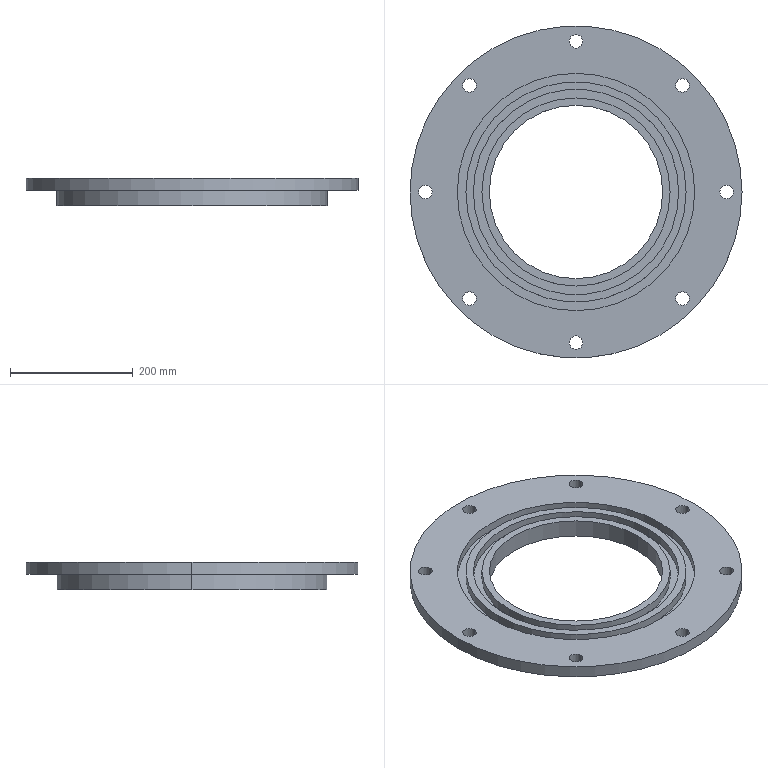Part | SolidWorks | features CirPattern 1, ICE 1, Revolution 1 | 1 solid | 40 faces | box 540 x 540 x 45 mm | volume 4136152 mm3 | cylinder 32 | plane 8 | commonest cylinder face diameters 22 x16 282 x2 306 x2 334 x2 358 x2 386 x2
STEP:
#1=CARTESIAN_POINT('',(-256.,0.,-20.));
#2=VERTEX_POINT('',#1);
#3=CARTESIAN_POINT('',(-234.,0.,-20.));
#4=VERTEX_POINT('',#3);
#5=CARTESIAN_POINT('',(-245.,0.,-20.));
#6=DIRECTION('',(0.,0.,1.));
#7=DIRECTION('',(1.,0.,0.));
#8=AXIS2_PLACEMENT_3D('',#5,#6,#7);
#9=CIRCLE('',#8,11.);
#10=EDGE_CURVE('',#2,#4,#9,.T.);
#11=ORIENTED_EDGE('',*,*,#10,.F.);
#12=CARTESIAN_POINT('',(-256.,0.,0.));
#13=VERTEX_POINT('',#12);
#14=CARTESIAN_POINT('',(-256.,0.,-41.));
#15=DIRECTION('',(0.,0.,1.));
#16=VECTOR('',#15,1000.);
#17=LINE('',#14,#16);
#18=EDGE_CURVE('',#2,#13,#17,.T.);
#19=ORIENTED_EDGE('',*,*,#18,.T.);
#20=CARTESIAN_POINT('',(-234.,0.,0.));
#21=VERTEX_POINT('',#20);
#22=CARTESIAN_POINT('',(-245.,0.,0.));
#23=DIRECTION('',(0.,0.,1.));
#24=DIRECTION('',(0.,1.,0.));
#25=AXIS2_PLACEMENT_3D('',#22,#23,#24);
#26=CIRCLE('',#25,11.);
#27=EDGE_CURVE('',#13,#21,#26,.T.);
#28=ORIENTED_EDGE('',*,*,#27,.T.);
#29=CARTESIAN_POINT('',(-234.,0.,-41.));
#30=DIRECTION('',(0.,0.,1.));
#31=VECTOR('',#30,1000.);
#32=LINE('',#29,#31);
#33=EDGE_CURVE('',#4,#21,#32,.T.);
#34=ORIENTED_EDGE('',*,*,#33,.F.);
#35=EDGE_LOOP('',(#11,#19,#28,#34));
#36=FACE_OUTER_BOUND('',#35,.T.);
#37=CARTESIAN_POINT('',(-245.,0.,-41.));
#38=DIRECTION('',(0.,0.,1.));
#39=DIRECTION('',(1.,0.,0.));
#40=AXIS2_PLACEMENT_3D('',#37,#38,#39);
#41=CYLINDRICAL_SURFACE('',#40,11.);
#42=ADVANCED_FACE('',(#36),#41,.F.);
#43=CARTESIAN_POINT('',(-184.241,-173.241,-20.));
#44=VERTEX_POINT('',#43);
#45=CARTESIAN_POINT('',(-162.241,-173.241,-20.));
#46=VERTEX_POINT('',#45);
#47=CARTESIAN_POINT('',(-173.241,-173.241,-20.));
#48=DIRECTION('',(0.,0.,1.));
#49=DIRECTION('',(1.,0.,0.));
#50=AXIS2_PLACEMENT_3D('',#47,#48,#49);
#51=CIRCLE('',#50,11.);
#52=EDGE_CURVE('',#44,#46,#51,.T.);
#53=ORIENTED_EDGE('',*,*,#52,.F.);
#54=CARTESIAN_POINT('',(-184.241,-173.241,0.));
#55=VERTEX_POINT('',#54);
#56=CARTESIAN_POINT('',(-184.241,-173.241,-41.));
#57=DIRECTION('',(0.,0.,1.));
#58=VECTOR('',#57,1000.);
#59=LINE('',#56,#58);
#60=EDGE_CURVE('',#44,#55,#59,.T.);
#61=ORIENTED_EDGE('',*,*,#60,.T.);
#62=CARTESIAN_POINT('',(-162.241,-173.241,0.));
#63=VERTEX_POINT('',#62);
#64=CARTESIAN_POINT('',(-173.241,-173.241,0.));
#65=DIRECTION('',(0.,0.,1.));
#66=DIRECTION('',(-0.7071,0.7071,0.));
#67=AXIS2_PLACEMENT_3D('',#64,#65,#66);
#68=CIRCLE('',#67,11.);
#69=EDGE_CURVE('',#55,#63,#68,.T.);
#70=ORIENTED_EDGE('',*,*,#69,.T.);
#71=CARTESIAN_POINT('',(-162.241,-173.241,-41.));
#72=DIRECTION('',(0.,0.,1.));
#73=VECTOR('',#72,1000.);
#74=LINE('',#71,#73);
#75=EDGE_CURVE('',#46,#63,#74,.T.);
#76=ORIENTED_EDGE('',*,*,#75,.F.);
#77=EDGE_LOOP('',(#53,#61,#70,#76));
#78=FACE_OUTER_BOUND('',#77,.T.);
#79=CARTESIAN_POINT('',(-173.241,-173.241,-41.));
#80=DIRECTION('',(0.,0.,1.));
#81=DIRECTION('',(1.,0.,0.));
#82=AXIS2_PLACEMENT_3D('',#79,#80,#81);
#83=CYLINDRICAL_SURFACE('',#82,11.);
#84=ADVANCED_FACE('',(#78),#83,.F.);
#85=CARTESIAN_POINT('',(-11.,-245.,-20.));
#86=VERTEX_POINT('',#85);
#87=CARTESIAN_POINT('',(11.,-245.,-20.));
#88=VERTEX_POINT('',#87);
#89=CARTESIAN_POINT('',(0.,-245.,-20.));
#90=DIRECTION('',(0.,0.,1.));
#91=DIRECTION('',(1.,0.,0.));
#92=AXIS2_PLACEMENT_3D('',#89,#90,#91);
#93=CIRCLE('',#92,11.);
#94=EDGE_CURVE('',#86,#88,#93,.T.);
#95=ORIENTED_EDGE('',*,*,#94,.F.);
#96=CARTESIAN_POINT('',(-11.,-245.,0.));
#97=VERTEX_POINT('',#96);
#98=CARTESIAN_POINT('',(-11.,-245.,-41.));
#99=DIRECTION('',(0.,0.,1.));
#100=VECTOR('',#99,1000.);
#101=LINE('',#98,#100);
#102=EDGE_CURVE('',#86,#97,#101,.T.);
#103=ORIENTED_EDGE('',*,*,#102,.T.);
#104=CARTESIAN_POINT('',(11.,-245.,0.));
#105=VERTEX_POINT('',#104);
#106=CARTESIAN_POINT('',(0.,-245.,0.));
#107=DIRECTION('',(0.,0.,1.));
#108=DIRECTION('',(-1.,0.,0.));
#109=AXIS2_PLACEMENT_3D('',#106,#107,#108);
#110=CIRCLE('',#109,11.);
#111=EDGE_CURVE('',#97,#105,#110,.T.);
#112=ORIENTED_EDGE('',*,*,#111,.T.);
#113=CARTESIAN_POINT('',(11.,-245.,-41.));
#114=DIRECTION('',(0.,0.,1.));
#115=VECTOR('',#114,1000.);
#116=LINE('',#113,#115);
#117=EDGE_CURVE('',#88,#105,#116,.T.);
#118=ORIENTED_EDGE('',*,*,#117,.F.);
#119=EDGE_LOOP('',(#95,#103,#112,#118));
#120=FACE_OUTER_BOUND('',#119,.T.);
#121=CARTESIAN_POINT('',(0.,-245.,-41.));
#122=DIRECTION('',(0.,0.,1.));
#123=DIRECTION('',(1.,0.,0.));
#124=AXIS2_PLACEMENT_3D('',#121,#122,#123);
#125=CYLINDRICAL_SURFACE('',#124,11.);
#126=ADVANCED_FACE('',(#120),#125,.F.);
#127=CARTESIAN_POINT('',(162.241,-173.241,-20.));
#128=VERTEX_POINT('',#127);
#129=CARTESIAN_POINT('',(184.241,-173.241,-20.));
#130=VERTEX_POINT('',#129);
#131=CARTESIAN_POINT('',(173.241,-173.241,-20.));
#132=DIRECTION('',(0.,0.,1.));
#133=DIRECTION('',(1.,0.,0.));
#134=AXIS2_PLACEMENT_3D('',#131,#132,#133);
#135=CIRCLE('',#134,11.);
#136=EDGE_CURVE('',#128,#130,#135,.T.);
#137=ORIENTED_EDGE('',*,*,#136,.F.);
#138=CARTESIAN_POINT('',(162.241,-173.241,0.));
#139=VERTEX_POINT('',#138);
#140=CARTESIAN_POINT('',(162.241,-173.241,-41.));
#141=DIRECTION('',(0.,0.,1.));
#142=VECTOR('',#141,1000.);
#143=LINE('',#140,#142);
#144=EDGE_CURVE('',#128,#139,#143,.T.);
#145=ORIENTED_EDGE('',*,*,#144,.T.);
#146=CARTESIAN_POINT('',(184.241,-173.241,0.));
#147=VERTEX_POINT('',#146);
#148=CARTESIAN_POINT('',(173.241,-173.241,0.));
#149=DIRECTION('',(0.,0.,1.));
#150=DIRECTION('',(-0.7071,-0.7071,0.));
#151=AXIS2_PLACEMENT_3D('',#148,#149,#150);
#152=CIRCLE('',#151,11.);
#153=EDGE_CURVE('',#139,#147,#152,.T.);
#154=ORIENTED_EDGE('',*,*,#153,.T.);
#155=CARTESIAN_POINT('',(184.241,-173.241,-41.));
#156=DIRECTION('',(0.,0.,1.));
#157=VECTOR('',#156,1000.);
#158=LINE('',#155,#157);
#159=EDGE_CURVE('',#130,#147,#158,.T.);
#160=ORIENTED_EDGE('',*,*,#159,.F.);
#161=EDGE_LOOP('',(#137,#145,#154,#160));
#162=FACE_OUTER_BOUND('',#161,.T.);
#163=CARTESIAN_POINT('',(173.241,-173.241,-41.));
#164=DIRECTION('',(0.,0.,1.));
#165=DIRECTION('',(1.,0.,0.));
#166=AXIS2_PLACEMENT_3D('',#163,#164,#165);
#167=CYLINDRICAL_SURFACE('',#166,11.);
#168=ADVANCED_FACE('',(#162),#167,.F.);
#169=CARTESIAN_POINT('',(234.,0.,-20.));
#170=VERTEX_POINT('',#169);
#171=CARTESIAN_POINT('',(256.,0.,-20.));
#172=VERTEX_POINT('',#171);
#173=CARTESIAN_POINT('',(245.,0.,-20.));
#174=DIRECTION('',(0.,0.,1.));
#175=DIRECTION('',(1.,0.,0.));
#176=AXIS2_PLACEMENT_3D('',#173,#174,#175);
#177=CIRCLE('',#176,11.);
#178=EDGE_CURVE('',#170,#172,#177,.T.);
#179=ORIENTED_EDGE('',*,*,#178,.F.);
#180=CARTESIAN_POINT('',(234.,0.,0.));
#181=VERTEX_POINT('',#180);
#182=CARTESIAN_POINT('',(234.,0.,-41.));
#183=DIRECTION('',(0.,0.,1.));
#184=VECTOR('',#183,1000.);
#185=LINE('',#182,#184);
#186=EDGE_CURVE('',#170,#181,#185,.T.);
#187=ORIENTED_EDGE('',*,*,#186,.T.);
#188=CARTESIAN_POINT('',(256.,0.,0.));
#189=VERTEX_POINT('',#188);
#190=CARTESIAN_POINT('',(245.,0.,0.));
#191=DIRECTION('',(0.,0.,1.));
#192=DIRECTION('',(0.,-1.,0.));
#193=AXIS2_PLACEMENT_3D('',#190,#191,#192);
#194=CIRCLE('',#193,11.);
#195=EDGE_CURVE('',#181,#189,#194,.T.);
#196=ORIENTED_EDGE('',*,*,#195,.T.);
#197=CARTESIAN_POINT('',(256.,0.,-41.));
#198=DIRECTION('',(0.,0.,1.));
#199=VECTOR('',#198,1000.);
#200=LINE('',#197,#199);
#201=EDGE_CURVE('',#172,#189,#200,.T.);
#202=ORIENTED_EDGE('',*,*,#201,.F.);
#203=EDGE_LOOP('',(#179,#187,#196,#202));
#204=FACE_OUTER_BOUND('',#203,.T.);
#205=CARTESIAN_POINT('',(245.,0.,-41.));
#206=DIRECTION('',(0.,0.,1.));
#207=DIRECTION('',(1.,0.,0.));
#208=AXIS2_PLACEMENT_3D('',#205,#206,#207);
#209=CYLINDRICAL_SURFACE('',#208,11.);
#210=ADVANCED_FACE('',(#204),#209,.F.);
#211=CARTESIAN_POINT('',(162.241,173.241,-20.));
#212=VERTEX_POINT('',#211);
#213=CARTESIAN_POINT('',(184.241,173.241,-20.));
#214=VERTEX_POINT('',#213);
#215=CARTESIAN_POINT('',(173.241,173.241,-20.));
#216=DIRECTION('',(0.,0.,1.));
#217=DIRECTION('',(1.,0.,0.));
#218=AXIS2_PLACEMENT_3D('',#215,#216,#217);
#219=CIRCLE('',#218,11.);
#220=EDGE_CURVE('',#212,#214,#219,.T.);
#221=ORIENTED_EDGE('',*,*,#220,.F.);
#222=CARTESIAN_POINT('',(162.241,173.241,0.));
#223=VERTEX_POINT('',#222);
#224=CARTESIAN_POINT('',(162.241,173.241,-41.));
#225=DIRECTION('',(0.,0.,1.));
#226=VECTOR('',#225,1000.);
#227=LINE('',#224,#226);
#228=EDGE_CURVE('',#212,#223,#227,.T.);
#229=ORIENTED_EDGE('',*,*,#228,.T.);
#230=CARTESIAN_POINT('',(184.241,173.241,0.));
#231=VERTEX_POINT('',#230);
#232=CARTESIAN_POINT('',(173.241,173.241,0.));
#233=DIRECTION('',(0.,0.,1.));
#234=DIRECTION('',(0.7071,-0.7071,0.));
#235=AXIS2_PLACEMENT_3D('',#232,#233,#234);
#236=CIRCLE('',#235,11.);
#237=EDGE_CURVE('',#223,#231,#236,.T.);
#238=ORIENTED_EDGE('',*,*,#237,.T.);
#239=CARTESIAN_POINT('',(184.241,173.241,-41.));
#240=DIRECTION('',(0.,0.,1.));
#241=VECTOR('',#240,1000.);
#242=LINE('',#239,#241);
#243=EDGE_CURVE('',#214,#231,#242,.T.);
#244=ORIENTED_EDGE('',*,*,#243,.F.);
#245=EDGE_LOOP('',(#221,#229,#238,#244));
#246=FACE_OUTER_BOUND('',#245,.T.);
#247=CARTESIAN_POINT('',(173.241,173.241,-41.));
#248=DIRECTION('',(0.,0.,1.));
#249=DIRECTION('',(1.,0.,0.));
#250=AXIS2_PLACEMENT_3D('',#247,#248,#249);
#251=CYLINDRICAL_SURFACE('',#250,11.);
#252=ADVANCED_FACE('',(#246),#251,.F.);
#253=CARTESIAN_POINT('',(-184.241,173.241,-20.));
#254=VERTEX_POINT('',#253);
#255=CARTESIAN_POINT('',(-162.241,173.241,-20.));
#256=VERTEX_POINT('',#255);
#257=CARTESIAN_POINT('',(-173.241,173.241,-20.));
#258=DIRECTION('',(0.,0.,1.));
#259=DIRECTION('',(1.,0.,0.));
#260=AXIS2_PLACEMENT_3D('',#257,#258,#259);
#261=CIRCLE('',#260,11.);
#262=EDGE_CURVE('',#254,#256,#261,.T.);
#263=ORIENTED_EDGE('',*,*,#262,.F.);
#264=CARTESIAN_POINT('',(-184.241,173.241,0.));
#265=VERTEX_POINT('',#264);
#266=CARTESIAN_POINT('',(-184.241,173.241,-41.));
#267=DIRECTION('',(0.,0.,1.));
#268=VECTOR('',#267,1000.);
#269=LINE('',#266,#268);
#270=EDGE_CURVE('',#254,#265,#269,.T.);
#271=ORIENTED_EDGE('',*,*,#270,.T.);
#272=CARTESIAN_POINT('',(-162.241,173.241,0.));
#273=VERTEX_POINT('',#272);
#274=CARTESIAN_POINT('',(-173.241,173.241,0.));
#275=DIRECTION('',(0.,0.,1.));
#276=DIRECTION('',(0.7071,0.7071,0.));
#277=AXIS2_PLACEMENT_3D('',#274,#275,#276);
#278=CIRCLE('',#277,11.);
#279=EDGE_CURVE('',#265,#273,#278,.T.);
#280=ORIENTED_EDGE('',*,*,#279,.T.);
#281=CARTESIAN_POINT('',(-162.241,173.241,-41.));
#282=DIRECTION('',(0.,0.,1.));
#283=VECTOR('',#282,1000.);
#284=LINE('',#281,#283);
#285=EDGE_CURVE('',#256,#273,#284,.T.);
#286=ORIENTED_EDGE('',*,*,#285,.F.);
#287=EDGE_LOOP('',(#263,#271,#280,#286));
#288=FACE_OUTER_BOUND('',#287,.T.);
#289=CARTESIAN_POINT('',(-173.241,173.241,-41.));
#290=DIRECTION('',(0.,0.,1.));
#291=DIRECTION('',(1.,0.,0.));
#292=AXIS2_PLACEMENT_3D('',#289,#290,#291);
#293=CYLINDRICAL_SURFACE('',#292,11.);
#294=ADVANCED_FACE('',(#288),#293,.F.);
#295=CARTESIAN_POINT('',(-11.,245.,-20.));
#296=VERTEX_POINT('',#295);
#297=CARTESIAN_POINT('',(11.,245.,-20.));
#298=VERTEX_POINT('',#297);
#299=CARTESIAN_POINT('',(0.,245.,-20.));
#300=DIRECTION('',(0.,0.,1.));
#301=DIRECTION('',(1.,0.,0.));
#302=AXIS2_PLACEMENT_3D('',#299,#300,#301);
#303=CIRCLE('',#302,11.);
#304=EDGE_CURVE('',#296,#298,#303,.T.);
#305=ORIENTED_EDGE('',*,*,#304,.F.);
#306=CARTESIAN_POINT('',(-11.,245.,0.));
#307=VERTEX_POINT('',#306);
#308=CARTESIAN_POINT('',(-11.,245.,-41.));
#309=DIRECTION('',(0.,0.,1.));
#310=VECTOR('',#309,1000.);
#311=LINE('',#308,#310);
#312=EDGE_CURVE('',#296,#307,#311,.T.);
#313=ORIENTED_EDGE('',*,*,#312,.T.);
#314=CARTESIAN_POINT('',(11.,245.,0.));
#315=VERTEX_POINT('',#314);
#316=CARTESIAN_POINT('',(0.,245.,0.));
#317=DIRECTION('',(0.,0.,1.));
#318=DIRECTION('',(1.,0.,0.));
#319=AXIS2_PLACEMENT_3D('',#316,#317,#318);
#320=CIRCLE('',#319,11.);
#321=EDGE_CURVE('',#307,#315,#320,.T.);
#322=ORIENTED_EDGE('',*,*,#321,.T.);
#323=CARTESIAN_POINT('',(11.,245.,-41.));
#324=DIRECTION('',(0.,0.,1.));
#325=VECTOR('',#324,1000.);
#326=LINE('',#323,#325);
#327=EDGE_CURVE('',#298,#315,#326,.T.);
#328=ORIENTED_EDGE('',*,*,#327,.F.);
#329=EDGE_LOOP('',(#305,#313,#322,#328));
#330=FACE_OUTER_BOUND('',#329,.T.);
#331=CARTESIAN_POINT('',(0.,245.,-41.));
#332=DIRECTION('',(0.,0.,1.));
#333=DIRECTION('',(1.,0.,0.));
#334=AXIS2_PLACEMENT_3D('',#331,#332,#333);
#335=CYLINDRICAL_SURFACE('',#334,11.);
#336=ADVANCED_FACE('',(#330),#335,.F.);
#337=CARTESIAN_POINT('',(-193.,0.,-14.));
#338=VERTEX_POINT('',#337);
#339=CARTESIAN_POINT('',(193.,0.,-14.));
#340=VERTEX_POINT('',#339);
#341=CARTESIAN_POINT('',(0.,0.,-14.));
#342=DIRECTION('',(0.,0.,1.));
#343=DIRECTION('',(1.,0.,0.));
#344=AXIS2_PLACEMENT_3D('',#341,#342,#343);
#345=CIRCLE('',#344,193.);
#346=EDGE_CURVE('',#338,#340,#345,.T.);
#347=ORIENTED_EDGE('',*,*,#346,.F.);
#348=CARTESIAN_POINT('',(-193.,0.,0.));
#349=VERTEX_POINT('',#348);
#350=CARTESIAN_POINT('',(-193.,0.,0.));
#351=DIRECTION('',(0.,0.,1.));
#352=VECTOR('',#351,1000.);
#353=LINE('',#350,#352);
#354=EDGE_CURVE('',#338,#349,#353,.T.);
#355=ORIENTED_EDGE('',*,*,#354,.T.);
#356=CARTESIAN_POINT('',(193.,0.,0.));
#357=VERTEX_POINT('',#356);
#358=CARTESIAN_POINT('',(0.,0.,0.));
#359=DIRECTION('',(0.,0.,1.));
#360=DIRECTION('',(1.,0.,0.));
#361=AXIS2_PLACEMENT_3D('',#358,#359,#360);
#362=CIRCLE('',#361,193.);
#363=EDGE_CURVE('',#349,#357,#362,.T.);
#364=ORIENTED_EDGE('',*,*,#363,.T.);
#365=CARTESIAN_POINT('',(193.,0.,0.));
#366=DIRECTION('',(0.,0.,1.));
#367=VECTOR('',#366,1000.);
#368=LINE('',#365,#367);
#369=EDGE_CURVE('',#340,#357,#368,.T.);
#370=ORIENTED_EDGE('',*,*,#369,.F.);
#371=EDGE_LOOP('',(#347,#355,#364,#370));
#372=FACE_OUTER_BOUND('',#371,.T.);
#373=CARTESIAN_POINT('',(0.,0.,0.));
#374=DIRECTION('',(0.,0.,1.));
#375=DIRECTION('',(1.,0.,0.));
#376=AXIS2_PLACEMENT_3D('',#373,#374,#375);
#377=CYLINDRICAL_SURFACE('',#376,193.);
#378=ADVANCED_FACE('',(#372),#377,.F.);
#379=CARTESIAN_POINT('',(179.,0.,-14.));
#380=VERTEX_POINT('',#379);
#381=CARTESIAN_POINT('',(-179.,0.,-14.));
#382=VERTEX_POINT('',#381);
#383=CARTESIAN_POINT('',(0.,0.,-14.));
#384=DIRECTION('',(0.,0.,1.));
#385=DIRECTION('',(1.,0.,0.));
#386=AXIS2_PLACEMENT_3D('',#383,#384,#385);
#387=CIRCLE('',#386,179.);
#388=EDGE_CURVE('',#380,#382,#387,.T.);
#389=ORIENTED_EDGE('',*,*,#388,.T.);
#390=CARTESIAN_POINT('',(-179.,0.,0.));
#391=VERTEX_POINT('',#390);
#392=CARTESIAN_POINT('',(-179.,0.,0.));
#393=DIRECTION('',(0.,0.,1.));
#394=VECTOR('',#393,1000.);
#395=LINE('',#392,#394);
#396=EDGE_CURVE('',#382,#391,#395,.T.);
#397=ORIENTED_EDGE('',*,*,#396,.T.);
#398=CARTESIAN_POINT('',(179.,0.,0.));
#399=VERTEX_POINT('',#398);
#400=CARTESIAN_POINT('',(0.,0.,0.));
#401=DIRECTION('',(0.,0.,1.));
#402=DIRECTION('',(1.,0.,0.));
#403=AXIS2_PLACEMENT_3D('',#400,#401,#402);
#404=CIRCLE('',#403,179.);
#405=EDGE_CURVE('',#399,#391,#404,.T.);
#406=ORIENTED_EDGE('',*,*,#405,.F.);
#407=CARTESIAN_POINT('',(179.,0.,0.));
#408=DIRECTION('',(0.,0.,1.));
#409=VECTOR('',#408,1000.);
#410=LINE('',#407,#409);
#411=EDGE_CURVE('',#380,#399,#410,.T.);
#412=ORIENTED_EDGE('',*,*,#411,.F.);
#413=EDGE_LOOP('',(#389,#397,#406,#412));
#414=FACE_OUTER_BOUND('',#413,.T.);
#415=CARTESIAN_POINT('',(0.,0.,0.));
#416=DIRECTION('',(0.,0.,1.));
#417=DIRECTION('',(1.,0.,0.));
#418=AXIS2_PLACEMENT_3D('',#415,#416,#417);
#419=CYLINDRICAL_SURFACE('',#418,179.);
#420=ADVANCED_FACE('',(#414),#419,.T.);
#421=CARTESIAN_POINT('',(-167.,0.,-14.));
#422=VERTEX_POINT('',#421);
#423=CARTESIAN_POINT('',(167.,0.,-14.));
#424=VERTEX_POINT('',#423);
#425=CARTESIAN_POINT('',(0.,0.,-14.));
#426=DIRECTION('',(0.,0.,1.));
#427=DIRECTION('',(1.,0.,0.));
#428=AXIS2_PLACEMENT_3D('',#425,#426,#427);
#429=CIRCLE('',#428,167.);
#430=EDGE_CURVE('',#422,#424,#429,.T.);
#431=ORIENTED_EDGE('',*,*,#430,.F.);
#432=CARTESIAN_POINT('',(-167.,0.,0.));
#433=VERTEX_POINT('',#432);
#434=CARTESIAN_POINT('',(-167.,0.,0.));
#435=DIRECTION('',(0.,0.,1.));
#436=VECTOR('',#435,1000.);
#437=LINE('',#434,#436);
#438=EDGE_CURVE('',#422,#433,#437,.T.);
#439=ORIENTED_EDGE('',*,*,#438,.T.);
#440=CARTESIAN_POINT('',(167.,0.,0.));
#441=VERTEX_POINT('',#440);
#442=CARTESIAN_POINT('',(0.,0.,0.));
#443=DIRECTION('',(0.,0.,1.));
#444=DIRECTION('',(1.,0.,0.));
#445=AXIS2_PLACEMENT_3D('',#442,#443,#444);
#446=CIRCLE('',#445,167.);
#447=EDGE_CURVE('',#433,#441,#446,.T.);
#448=ORIENTED_EDGE('',*,*,#447,.T.);
#449=CARTESIAN_POINT('',(167.,0.,0.));
#450=DIRECTION('',(0.,0.,1.));
#451=VECTOR('',#450,1000.);
#452=LINE('',#449,#451);
#453=EDGE_CURVE('',#424,#441,#452,.T.);
#454=ORIENTED_EDGE('',*,*,#453,.F.);
#455=EDGE_LOOP('',(#431,#439,#448,#454));
#456=FACE_OUTER_BOUND('',#455,.T.);
#457=CARTESIAN_POINT('',(0.,0.,0.));
#458=DIRECTION('',(0.,0.,1.));
#459=DIRECTION('',(1.,0.,0.));
#460=AXIS2_PLACEMENT_3D('',#457,#458,#459);
#461=CYLINDRICAL_SURFACE('',#460,167.);
#462=ADVANCED_FACE('',(#456),#461,.F.);
#463=CARTESIAN_POINT('',(153.,0.,-14.));
#464=VERTEX_POINT('',#463);
#465=CARTESIAN_POINT('',(-153.,0.,-14.));
#466=VERTEX_POINT('',#465);
#467=CARTESIAN_POINT('',(0.,0.,-14.));
#468=DIRECTION('',(0.,0.,1.));
#469=DIRECTION('',(1.,0.,0.));
#470=AXIS2_PLACEMENT_3D('',#467,#468,#469);
#471=CIRCLE('',#470,153.);
#472=EDGE_CURVE('',#464,#466,#471,.T.);
#473=ORIENTED_EDGE('',*,*,#472,.T.);
#474=CARTESIAN_POINT('',(-153.,0.,0.));
#475=VERTEX_POINT('',#474);
#476=CARTESIAN_POINT('',(-153.,0.,0.));
#477=DIRECTION('',(0.,0.,1.));
#478=VECTOR('',#477,1000.);
#479=LINE('',#476,#478);
#480=EDGE_CURVE('',#466,#475,#479,.T.);
#481=ORIENTED_EDGE('',*,*,#480,.T.);
#482=CARTESIAN_POINT('',(153.,0.,0.));
#483=VERTEX_POINT('',#482);
#484=CARTESIAN_POINT('',(0.,0.,0.));
#485=DIRECTION('',(0.,0.,1.));
#486=DIRECTION('',(1.,0.,0.));
#487=AXIS2_PLACEMENT_3D('',#484,#485,#486);
#488=CIRCLE('',#487,153.);
#489=EDGE_CURVE('',#483,#475,#488,.T.);
#490=ORIENTED_EDGE('',*,*,#489,.F.);
#491=CARTESIAN_POINT('',(153.,0.,0.));
#492=DIRECTION('',(0.,0.,1.));
#493=VECTOR('',#492,1000.);
#494=LINE('',#491,#493);
#495=EDGE_CURVE('',#464,#483,#494,.T.);
#496=ORIENTED_EDGE('',*,*,#495,.F.);
#497=EDGE_LOOP('',(#473,#481,#490,#496));
#498=FACE_OUTER_BOUND('',#497,.T.);
#499=CARTESIAN_POINT('',(0.,0.,0.));
#500=DIRECTION('',(0.,0.,1.));
#501=DIRECTION('',(1.,0.,0.));
#502=AXIS2_PLACEMENT_3D('',#499,#500,#501);
#503=CYLINDRICAL_SURFACE('',#502,153.);
#504=ADVANCED_FACE('',(#498),#503,.T.);
#505=CARTESIAN_POINT('',(-141.,0.,-30.));
#506=VERTEX_POINT('',#505);
#507=CARTESIAN_POINT('',(141.,0.,-30.));
#508=VERTEX_POINT('',#507);
#509=CARTESIAN_POINT('',(0.,0.,-30.));
#510=DIRECTION('',(0.,0.,1.));
#511=DIRECTION('',(1.,0.,0.));
#512=AXIS2_PLACEMENT_3D('',#509,#510,#511);
#513=CIRCLE('',#512,141.);
#514=EDGE_CURVE('',#506,#508,#513,.T.);
#515=ORIENTED_EDGE('',*,*,#514,.F.);
#516=CARTESIAN_POINT('',(-141.,0.,0.));
#517=VERTEX_POINT('',#516);
#518=CARTESIAN_POINT('',(-141.,0.,0.));
#519=DIRECTION('',(0.,0.,1.));
#520=VECTOR('',#519,1000.);
#521=LINE('',#518,#520);
#522=EDGE_CURVE('',#506,#517,#521,.T.);
#523=ORIENTED_EDGE('',*,*,#522,.T.);
#524=CARTESIAN_POINT('',(141.,0.,0.));
#525=VERTEX_POINT('',#524);
#526=CARTESIAN_POINT('',(0.,0.,0.));
#527=DIRECTION('',(0.,0.,1.));
#528=DIRECTION('',(1.,0.,0.));
#529=AXIS2_PLACEMENT_3D('',#526,#527,#528);
#530=CIRCLE('',#529,141.);
#531=EDGE_CURVE('',#517,#525,#530,.T.);
#532=ORIENTED_EDGE('',*,*,#531,.T.);
#533=CARTESIAN_POINT('',(141.,0.,0.));
#534=DIRECTION('',(0.,0.,1.));
#535=VECTOR('',#534,1000.);
#536=LINE('',#533,#535);
#537=EDGE_CURVE('',#508,#525,#536,.T.);
#538=ORIENTED_EDGE('',*,*,#537,.F.);
#539=EDGE_LOOP('',(#515,#523,#532,#538));
#540=FACE_OUTER_BOUND('',#539,.T.);
#541=CARTESIAN_POINT('',(0.,0.,0.));
#542=DIRECTION('',(0.,0.,1.));
#543=DIRECTION('',(1.,0.,0.));
#544=AXIS2_PLACEMENT_3D('',#541,#542,#543);
#545=CYLINDRICAL_SURFACE('',#544,141.);
#546=ADVANCED_FACE('',(#540),#545,.F.);
#547=CARTESIAN_POINT('',(-200.,0.,-45.));
#548=VERTEX_POINT('',#547);
#549=CARTESIAN_POINT('',(200.,0.,-45.));
#550=VERTEX_POINT('',#549);
#551=CARTESIAN_POINT('',(0.,0.,-45.));
#552=DIRECTION('',(0.,0.,1.));
#553=DIRECTION('',(1.,0.,0.));
#554=AXIS2_PLACEMENT_3D('',#551,#552,#553);
#555=CIRCLE('',#554,200.);
#556=EDGE_CURVE('',#548,#550,#555,.T.);
#557=ORIENTED_EDGE('',*,*,#556,.F.);
#558=CARTESIAN_POINT('',(-200.,0.,-30.));
#559=VERTEX_POINT('',#558);
#560=CARTESIAN_POINT('',(-200.,0.,0.));
#561=DIRECTION('',(0.,0.,1.));
#562=VECTOR('',#561,1000.);
#563=LINE('',#560,#562);
#564=EDGE_CURVE('',#548,#559,#563,.T.);
#565=ORIENTED_EDGE('',*,*,#564,.T.);
#566=CARTESIAN_POINT('',(200.,0.,-30.));
#567=VERTEX_POINT('',#566);
#568=CARTESIAN_POINT('',(0.,0.,-30.));
#569=DIRECTION('',(0.,0.,1.));
#570=DIRECTION('',(1.,0.,0.));
#571=AXIS2_PLACEMENT_3D('',#568,#569,#570);
#572=CIRCLE('',#571,200.);
#573=EDGE_CURVE('',#559,#567,#572,.T.);
#574=ORIENTED_EDGE('',*,*,#573,.T.);
#575=CARTESIAN_POINT('',(200.,0.,0.));
#576=DIRECTION('',(0.,0.,1.));
#577=VECTOR('',#576,1000.);
#578=LINE('',#575,#577);
#579=EDGE_CURVE('',#550,#567,#578,.T.);
#580=ORIENTED_EDGE('',*,*,#579,.F.);
#581=EDGE_LOOP('',(#557,#565,#574,#580));
#582=FACE_OUTER_BOUND('',#581,.T.);
#583=CARTESIAN_POINT('',(0.,0.,0.));
#584=DIRECTION('',(0.,0.,1.));
#585=DIRECTION('',(1.,0.,0.));
#586=AXIS2_PLACEMENT_3D('',#583,#584,#585);
#587=CYLINDRICAL_SURFACE('',#586,200.);
#588=ADVANCED_FACE('',(#582),#587,.F.);
#589=CARTESIAN_POINT('',(220.,0.,-45.));
#590=VERTEX_POINT('',#589);
#591=CARTESIAN_POINT('',(-220.,0.,-45.));
#592=VERTEX_POINT('',#591);
#593=CARTESIAN_POINT('',(0.,0.,-45.));
#594=DIRECTION('',(0.,0.,1.));
#595=DIRECTION('',(1.,0.,0.));
#596=AXIS2_PLACEMENT_3D('',#593,#594,#595);
#597=CIRCLE('',#596,220.);
#598=EDGE_CURVE('',#590,#592,#597,.T.);
#599=ORIENTED_EDGE('',*,*,#598,.T.);
#600=CARTESIAN_POINT('',(-220.,0.,-20.));
#601=VERTEX_POINT('',#600);
#602=CARTESIAN_POINT('',(-220.,0.,0.));
#603=DIRECTION('',(0.,0.,1.));
#604=VECTOR('',#603,1000.);
#605=LINE('',#602,#604);
#606=EDGE_CURVE('',#592,#601,#605,.T.);
#607=ORIENTED_EDGE('',*,*,#606,.T.);
#608=CARTESIAN_POINT('',(220.,0.,-20.));
#609=VERTEX_POINT('',#608);
#610=CARTESIAN_POINT('',(0.,0.,-20.));
#611=DIRECTION('',(0.,0.,1.));
#612=DIRECTION('',(1.,0.,0.));
#613=AXIS2_PLACEMENT_3D('',#610,#611,#612);
#614=CIRCLE('',#613,220.);
#615=EDGE_CURVE('',#609,#601,#614,.T.);
#616=ORIENTED_EDGE('',*,*,#615,.F.);
#617=CARTESIAN_POINT('',(220.,0.,0.));
#618=DIRECTION('',(0.,0.,1.));
#619=VECTOR('',#618,1000.);
#620=LINE('',#617,#619);
#621=EDGE_CURVE('',#590,#609,#620,.T.);
#622=ORIENTED_EDGE('',*,*,#621,.F.);
#623=EDGE_LOOP('',(#599,#607,#616,#622));
#624=FACE_OUTER_BOUND('',#623,.T.);
#625=CARTESIAN_POINT('',(0.,0.,0.));
#626=DIRECTION('',(0.,0.,1.));
#627=DIRECTION('',(1.,0.,0.));
#628=AXIS2_PLACEMENT_3D('',#625,#626,#627);
#629=CYLINDRICAL_SURFACE('',#628,220.);
#630=ADVANCED_FACE('',(#624),#629,.T.);
#631=CARTESIAN_POINT('',(270.,0.,-20.));
#632=VERTEX_POINT('',#631);
#633=CARTESIAN_POINT('',(-270.,0.,-20.));
#634=VERTEX_POINT('',#633);
#635=CARTESIAN_POINT('',(0.,0.,-20.));
#636=DIRECTION('',(0.,0.,1.));
#637=DIRECTION('',(1.,0.,0.));
#638=AXIS2_PLACEMENT_3D('',#635,#636,#637);
#639=CIRCLE('',#638,270.);
#640=EDGE_CURVE('',#632,#634,#639,.T.);
#641=ORIENTED_EDGE('',*,*,#640,.T.);
#642=CARTESIAN_POINT('',(-270.,0.,0.));
#643=VERTEX_POINT('',#642);
#644=CARTESIAN_POINT('',(-270.,0.,0.));
#645=DIRECTION('',(0.,0.,1.));
#646=VECTOR('',#645,1000.);
#647=LINE('',#644,#646);
#648=EDGE_CURVE('',#634,#643,#647,.T.);
#649=ORIENTED_EDGE('',*,*,#648,.T.);
#650=CARTESIAN_POINT('',(270.,0.,0.));
#651=VERTEX_POINT('',#650);
#652=CARTESIAN_POINT('',(0.,0.,0.));
#653=DIRECTION('',(0.,0.,1.));
#654=DIRECTION('',(1.,0.,0.));
#655=AXIS2_PLACEMENT_3D('',#652,#653,#654);
#656=CIRCLE('',#655,270.);
#657=EDGE_CURVE('',#651,#643,#656,.T.);
#658=ORIENTED_EDGE('',*,*,#657,.F.);
#659=CARTESIAN_POINT('',(270.,0.,0.));
#660=DIRECTION('',(0.,0.,1.));
#661=VECTOR('',#660,1000.);
#662=LINE('',#659,#661);
#663=EDGE_CURVE('',#632,#651,#662,.T.);
#664=ORIENTED_EDGE('',*,*,#663,.F.);
#665=EDGE_LOOP('',(#641,#649,#658,#664));
#666=FACE_OUTER_BOUND('',#665,.T.);
#667=CARTESIAN_POINT('',(0.,0.,0.));
#668=DIRECTION('',(0.,0.,1.));
#669=DIRECTION('',(1.,0.,0.));
#670=AXIS2_PLACEMENT_3D('',#667,#668,#669);
#671=CYLINDRICAL_SURFACE('',#670,270.);
#672=ADVANCED_FACE('',(#666),#671,.T.);
#673=CARTESIAN_POINT('',(-245.,0.,0.));
#674=DIRECTION('',(0.,0.,1.));
#675=DIRECTION('',(0.,1.,0.));
#676=AXIS2_PLACEMENT_3D('',#673,#674,#675);
#677=CIRCLE('',#676,11.);
#678=EDGE_CURVE('',#21,#13,#677,.T.);
#679=ORIENTED_EDGE('',*,*,#678,.F.);
#680=ORIENTED_EDGE('',*,*,#27,.F.);
#681=EDGE_LOOP('',(#679,#680));
#682=FACE_BOUND('',#681,.T.);
#683=CARTESIAN_POINT('',(-173.241,-173.241,0.));
#684=DIRECTION('',(0.,0.,1.));
#685=DIRECTION('',(-0.7071,0.7071,0.));
#686=AXIS2_PLACEMENT_3D('',#683,#684,#685);
#687=CIRCLE('',#686,11.);
#688=EDGE_CURVE('',#63,#55,#687,.T.);
#689=ORIENTED_EDGE('',*,*,#688,.F.);
#690=ORIENTED_EDGE('',*,*,#69,.F.);
#691=EDGE_LOOP('',(#689,#690));
#692=FACE_BOUND('',#691,.T.);
#693=CARTESIAN_POINT('',(0.,-245.,0.));
#694=DIRECTION('',(0.,0.,1.));
#695=DIRECTION('',(-1.,0.,0.));
#696=AXIS2_PLACEMENT_3D('',#693,#694,#695);
#697=CIRCLE('',#696,11.);
#698=EDGE_CURVE('',#105,#97,#697,.T.);
#699=ORIENTED_EDGE('',*,*,#698,.F.);
#700=ORIENTED_EDGE('',*,*,#111,.F.);
#701=EDGE_LOOP('',(#699,#700));
#702=FACE_BOUND('',#701,.T.);
#703=CARTESIAN_POINT('',(173.241,-173.241,0.));
#704=DIRECTION('',(0.,0.,1.));
#705=DIRECTION('',(-0.7071,-0.7071,0.));
#706=AXIS2_PLACEMENT_3D('',#703,#704,#705);
#707=CIRCLE('',#706,11.);
#708=EDGE_CURVE('',#147,#139,#707,.T.);
#709=ORIENTED_EDGE('',*,*,#708,.F.);
#710=ORIENTED_EDGE('',*,*,#153,.F.);
#711=EDGE_LOOP('',(#709,#710));
#712=FACE_BOUND('',#711,.T.);
#713=CARTESIAN_POINT('',(245.,0.,0.));
#714=DIRECTION('',(0.,0.,1.));
#715=DIRECTION('',(0.,-1.,0.));
#716=AXIS2_PLACEMENT_3D('',#713,#714,#715);
#717=CIRCLE('',#716,11.);
#718=EDGE_CURVE('',#189,#181,#717,.T.);
#719=ORIENTED_EDGE('',*,*,#718,.F.);
#720=ORIENTED_EDGE('',*,*,#195,.F.);
#721=EDGE_LOOP('',(#719,#720));
#722=FACE_BOUND('',#721,.T.);
#723=CARTESIAN_POINT('',(173.241,173.241,0.));
#724=DIRECTION('',(0.,0.,1.));
#725=DIRECTION('',(0.7071,-0.7071,0.));
#726=AXIS2_PLACEMENT_3D('',#723,#724,#725);
#727=CIRCLE('',#726,11.);
#728=EDGE_CURVE('',#231,#223,#727,.T.);
#729=ORIENTED_EDGE('',*,*,#728,.F.);
#730=ORIENTED_EDGE('',*,*,#237,.F.);
#731=EDGE_LOOP('',(#729,#730));
#732=FACE_BOUND('',#731,.T.);
#733=CARTESIAN_POINT('',(-173.241,173.241,0.));
#734=DIRECTION('',(0.,0.,1.));
#735=DIRECTION('',(0.7071,0.7071,0.));
#736=AXIS2_PLACEMENT_3D('',#733,#734,#735);
#737=CIRCLE('',#736,11.);
#738=EDGE_CURVE('',#273,#265,#737,.T.);
#739=ORIENTED_EDGE('',*,*,#738,.F.);
#740=ORIENTED_EDGE('',*,*,#279,.F.);
#741=EDGE_LOOP('',(#739,#740));
#742=FACE_BOUND('',#741,.T.);
#743=CARTESIAN_POINT('',(0.,245.,0.));
#744=DIRECTION('',(0.,0.,1.));
#745=DIRECTION('',(1.,0.,0.));
#746=AXIS2_PLACEMENT_3D('',#743,#744,#745);
#747=CIRCLE('',#746,11.);
#748=EDGE_CURVE('',#315,#307,#747,.T.);
#749=ORIENTED_EDGE('',*,*,#748,.F.);
#750=ORIENTED_EDGE('',*,*,#321,.F.);
#751=EDGE_LOOP('',(#749,#750));
#752=FACE_BOUND('',#751,.T.);
#753=CARTESIAN_POINT('',(0.,0.,0.));
#754=DIRECTION('',(0.,0.,1.));
#755=DIRECTION('',(1.,0.,0.));
#756=AXIS2_PLACEMENT_3D('',#753,#754,#755);
#757=CIRCLE('',#756,193.);
#758=EDGE_CURVE('',#357,#349,#757,.T.);
#759=ORIENTED_EDGE('',*,*,#758,.F.);
#760=ORIENTED_EDGE('',*,*,#363,.F.);
#761=EDGE_LOOP('',(#759,#760));
#762=FACE_BOUND('',#761,.T.);
#763=ORIENTED_EDGE('',*,*,#657,.T.);
#764=CARTESIAN_POINT('',(0.,0.,0.));
#765=DIRECTION('',(0.,0.,1.));
#766=DIRECTION('',(1.,0.,0.));
#767=AXIS2_PLACEMENT_3D('',#764,#765,#766);
#768=CIRCLE('',#767,270.);
#769=EDGE_CURVE('',#643,#651,#768,.T.);
#770=ORIENTED_EDGE('',*,*,#769,.T.);
#771=EDGE_LOOP('',(#763,#770));
#772=FACE_OUTER_BOUND('',#771,.T.);
#773=CARTESIAN_POINT('',(0.,193.,0.));
#774=DIRECTION('',(0.,0.,-1.));
#775=DIRECTION('',(-1.,0.,0.));
#776=AXIS2_PLACEMENT_3D('',#773,#774,#775);
#777=PLANE('',#776);
#778=ADVANCED_FACE('',(#682,#692,#702,#712,#722,#732,#742,#752,#762,#772),#777,.F.);
#779=ORIENTED_EDGE('',*,*,#648,.F.);
#780=CARTESIAN_POINT('',(0.,0.,-20.));
#781=DIRECTION('',(0.,0.,1.));
#782=DIRECTION('',(1.,0.,0.));
#783=AXIS2_PLACEMENT_3D('',#780,#781,#782);
#784=CIRCLE('',#783,270.);
#785=EDGE_CURVE('',#634,#632,#784,.T.);
#786=ORIENTED_EDGE('',*,*,#785,.T.);
#787=ORIENTED_EDGE('',*,*,#663,.T.);
#788=ORIENTED_EDGE('',*,*,#769,.F.);
#789=EDGE_LOOP('',(#779,#786,#787,#788));
#790=FACE_OUTER_BOUND('',#789,.T.);
#791=CARTESIAN_POINT('',(0.,0.,0.));
#792=DIRECTION('',(0.,0.,1.));
#793=DIRECTION('',(1.,0.,0.));
#794=AXIS2_PLACEMENT_3D('',#791,#792,#793);
#795=CYLINDRICAL_SURFACE('',#794,270.);
#796=ADVANCED_FACE('',(#790),#795,.T.);
#797=CARTESIAN_POINT('',(-245.,0.,-20.));
#798=DIRECTION('',(0.,0.,1.));
#799=DIRECTION('',(1.,0.,0.));
#800=AXIS2_PLACEMENT_3D('',#797,#798,#799);
#801=CIRCLE('',#800,11.);
#802=EDGE_CURVE('',#4,#2,#801,.T.);
#803=ORIENTED_EDGE('',*,*,#802,.T.);
#804=ORIENTED_EDGE('',*,*,#10,.T.);
#805=EDGE_LOOP('',(#803,#804));
#806=FACE_BOUND('',#805,.T.);
#807=CARTESIAN_POINT('',(-173.241,-173.241,-20.));
#808=DIRECTION('',(0.,0.,1.));
#809=DIRECTION('',(1.,0.,0.));
#810=AXIS2_PLACEMENT_3D('',#807,#808,#809);
#811=CIRCLE('',#810,11.);
#812=EDGE_CURVE('',#46,#44,#811,.T.);
#813=ORIENTED_EDGE('',*,*,#812,.T.);
#814=ORIENTED_EDGE('',*,*,#52,.T.);
#815=EDGE_LOOP('',(#813,#814));
#816=FACE_BOUND('',#815,.T.);
#817=CARTESIAN_POINT('',(0.,-245.,-20.));
#818=DIRECTION('',(0.,0.,1.));
#819=DIRECTION('',(1.,0.,0.));
#820=AXIS2_PLACEMENT_3D('',#817,#818,#819);
#821=CIRCLE('',#820,11.);
#822=EDGE_CURVE('',#88,#86,#821,.T.);
#823=ORIENTED_EDGE('',*,*,#822,.T.);
#824=ORIENTED_EDGE('',*,*,#94,.T.);
#825=EDGE_LOOP('',(#823,#824));
#826=FACE_BOUND('',#825,.T.);
#827=CARTESIAN_POINT('',(173.241,-173.241,-20.));
#828=DIRECTION('',(0.,0.,1.));
#829=DIRECTION('',(1.,0.,0.));
#830=AXIS2_PLACEMENT_3D('',#827,#828,#829);
#831=CIRCLE('',#830,11.);
#832=EDGE_CURVE('',#130,#128,#831,.T.);
#833=ORIENTED_EDGE('',*,*,#832,.T.);
#834=ORIENTED_EDGE('',*,*,#136,.T.);
#835=EDGE_LOOP('',(#833,#834));
#836=FACE_BOUND('',#835,.T.);
#837=CARTESIAN_POINT('',(245.,0.,-20.));
#838=DIRECTION('',(0.,0.,1.));
#839=DIRECTION('',(1.,0.,0.));
#840=AXIS2_PLACEMENT_3D('',#837,#838,#839);
#841=CIRCLE('',#840,11.);
#842=EDGE_CURVE('',#172,#170,#841,.T.);
#843=ORIENTED_EDGE('',*,*,#842,.T.);
#844=ORIENTED_EDGE('',*,*,#178,.T.);
#845=EDGE_LOOP('',(#843,#844));
#846=FACE_BOUND('',#845,.T.);
#847=CARTESIAN_POINT('',(173.241,173.241,-20.));
#848=DIRECTION('',(0.,0.,1.));
#849=DIRECTION('',(1.,0.,0.));
#850=AXIS2_PLACEMENT_3D('',#847,#848,#849);
#851=CIRCLE('',#850,11.);
#852=EDGE_CURVE('',#214,#212,#851,.T.);
#853=ORIENTED_EDGE('',*,*,#852,.T.);
#854=ORIENTED_EDGE('',*,*,#220,.T.);
#855=EDGE_LOOP('',(#853,#854));
#856=FACE_BOUND('',#855,.T.);
#857=CARTESIAN_POINT('',(-173.241,173.241,-20.));
#858=DIRECTION('',(0.,0.,1.));
#859=DIRECTION('',(1.,0.,0.));
#860=AXIS2_PLACEMENT_3D('',#857,#858,#859);
#861=CIRCLE('',#860,11.);
#862=EDGE_CURVE('',#256,#254,#861,.T.);
#863=ORIENTED_EDGE('',*,*,#862,.T.);
#864=ORIENTED_EDGE('',*,*,#262,.T.);
#865=EDGE_LOOP('',(#863,#864));
#866=FACE_BOUND('',#865,.T.);
#867=CARTESIAN_POINT('',(0.,245.,-20.));
#868=DIRECTION('',(0.,0.,1.));
#869=DIRECTION('',(1.,0.,0.));
#870=AXIS2_PLACEMENT_3D('',#867,#868,#869);
#871=CIRCLE('',#870,11.);
#872=EDGE_CURVE('',#298,#296,#871,.T.);
#873=ORIENTED_EDGE('',*,*,#872,.T.);
#874=ORIENTED_EDGE('',*,*,#304,.T.);
#875=EDGE_LOOP('',(#873,#874));
#876=FACE_BOUND('',#875,.T.);
#877=ORIENTED_EDGE('',*,*,#640,.F.);
#878=ORIENTED_EDGE('',*,*,#785,.F.);
#879=EDGE_LOOP('',(#877,#878));
#880=FACE_OUTER_BOUND('',#879,.T.);
#881=ORIENTED_EDGE('',*,*,#615,.T.);
#882=CARTESIAN_POINT('',(0.,0.,-20.));
#883=DIRECTION('',(0.,0.,1.));
#884=DIRECTION('',(1.,0.,0.));
#885=AXIS2_PLACEMENT_3D('',#882,#883,#884);
#886=CIRCLE('',#885,220.);
#887=EDGE_CURVE('',#601,#609,#886,.T.);
#888=ORIENTED_EDGE('',*,*,#887,.T.);
#889=EDGE_LOOP('',(#881,#888));
#890=FACE_BOUND('',#889,.T.);
#891=CARTESIAN_POINT('',(0.,270.,-20.));
#892=DIRECTION('',(0.,0.,1.));
#893=DIRECTION('',(1.,0.,0.));
#894=AXIS2_PLACEMENT_3D('',#891,#892,#893);
#895=PLANE('',#894);
#896=ADVANCED_FACE('',(#806,#816,#826,#836,#846,#856,#866,#876,#880,#890),#895,.F.);
#897=ORIENTED_EDGE('',*,*,#606,.F.);
#898=CARTESIAN_POINT('',(0.,0.,-45.));
#899=DIRECTION('',(0.,0.,1.));
#900=DIRECTION('',(1.,0.,0.));
#901=AXIS2_PLACEMENT_3D('',#898,#899,#900);
#902=CIRCLE('',#901,220.);
#903=EDGE_CURVE('',#592,#590,#902,.T.);
#904=ORIENTED_EDGE('',*,*,#903,.T.);
#905=ORIENTED_EDGE('',*,*,#621,.T.);
#906=ORIENTED_EDGE('',*,*,#887,.F.);
#907=EDGE_LOOP('',(#897,#904,#905,#906));
#908=FACE_OUTER_BOUND('',#907,.T.);
#909=CARTESIAN_POINT('',(0.,0.,0.));
#910=DIRECTION('',(0.,0.,1.));
#911=DIRECTION('',(1.,0.,0.));
#912=AXIS2_PLACEMENT_3D('',#909,#910,#911);
#913=CYLINDRICAL_SURFACE('',#912,220.);
#914=ADVANCED_FACE('',(#908),#913,.T.);
#915=ORIENTED_EDGE('',*,*,#598,.F.);
#916=ORIENTED_EDGE('',*,*,#903,.F.);
#917=EDGE_LOOP('',(#915,#916));
#918=FACE_OUTER_BOUND('',#917,.T.);
#919=CARTESIAN_POINT('',(0.,0.,-45.));
#920=DIRECTION('',(0.,0.,1.));
#921=DIRECTION('',(1.,0.,0.));
#922=AXIS2_PLACEMENT_3D('',#919,#920,#921);
#923=CIRCLE('',#922,200.);
#924=EDGE_CURVE('',#550,#548,#923,.T.);
#925=ORIENTED_EDGE('',*,*,#924,.T.);
#926=ORIENTED_EDGE('',*,*,#556,.T.);
#927=EDGE_LOOP('',(#925,#926));
#928=FACE_BOUND('',#927,.T.);
#929=CARTESIAN_POINT('',(0.,220.,-45.));
#930=DIRECTION('',(0.,0.,1.));
#931=DIRECTION('',(1.,0.,0.));
#932=AXIS2_PLACEMENT_3D('',#929,#930,#931);
#933=PLANE('',#932);
#934=ADVANCED_FACE('',(#918,#928),#933,.F.);
#935=ORIENTED_EDGE('',*,*,#564,.F.);
#936=ORIENTED_EDGE('',*,*,#924,.F.);
#937=ORIENTED_EDGE('',*,*,#579,.T.);
#938=CARTESIAN_POINT('',(0.,0.,-30.));
#939=DIRECTION('',(0.,0.,1.));
#940=DIRECTION('',(1.,0.,0.));
#941=AXIS2_PLACEMENT_3D('',#938,#939,#940);
#942=CIRCLE('',#941,200.);
#943=EDGE_CURVE('',#567,#559,#942,.T.);
#944=ORIENTED_EDGE('',*,*,#943,.T.);
#945=EDGE_LOOP('',(#935,#936,#937,#944));
#946=FACE_OUTER_BOUND('',#945,.T.);
#947=CARTESIAN_POINT('',(0.,0.,0.));
#948=DIRECTION('',(0.,0.,1.));
#949=DIRECTION('',(1.,0.,0.));
#950=AXIS2_PLACEMENT_3D('',#947,#948,#949);
#951=CYLINDRICAL_SURFACE('',#950,200.);
#952=ADVANCED_FACE('',(#946),#951,.F.);
#953=ORIENTED_EDGE('',*,*,#943,.F.);
#954=ORIENTED_EDGE('',*,*,#573,.F.);
#955=EDGE_LOOP('',(#953,#954));
#956=FACE_OUTER_BOUND('',#955,.T.);
#957=CARTESIAN_POINT('',(0.,0.,-30.));
#958=DIRECTION('',(0.,0.,1.));
#959=DIRECTION('',(1.,0.,0.));
#960=AXIS2_PLACEMENT_3D('',#957,#958,#959);
#961=CIRCLE('',#960,141.);
#962=EDGE_CURVE('',#508,#506,#961,.T.);
#963=ORIENTED_EDGE('',*,*,#962,.T.);
#964=ORIENTED_EDGE('',*,*,#514,.T.);
#965=EDGE_LOOP('',(#963,#964));
#966=FACE_BOUND('',#965,.T.);
#967=CARTESIAN_POINT('',(0.,200.,-30.));
#968=DIRECTION('',(0.,0.,1.));
#969=DIRECTION('',(1.,0.,0.));
#970=AXIS2_PLACEMENT_3D('',#967,#968,#969);
#971=PLANE('',#970);
#972=ADVANCED_FACE('',(#956,#966),#971,.F.);
#973=ORIENTED_EDGE('',*,*,#522,.F.);
#974=ORIENTED_EDGE('',*,*,#962,.F.);
#975=ORIENTED_EDGE('',*,*,#537,.T.);
#976=CARTESIAN_POINT('',(0.,0.,0.));
#977=DIRECTION('',(0.,0.,1.));
#978=DIRECTION('',(1.,0.,0.));
#979=AXIS2_PLACEMENT_3D('',#976,#977,#978);
#980=CIRCLE('',#979,141.);
#981=EDGE_CURVE('',#525,#517,#980,.T.);
#982=ORIENTED_EDGE('',*,*,#981,.T.);
#983=EDGE_LOOP('',(#973,#974,#975,#982));
#984=FACE_OUTER_BOUND('',#983,.T.);
#985=CARTESIAN_POINT('',(0.,0.,0.));
#986=DIRECTION('',(0.,0.,1.));
#987=DIRECTION('',(1.,0.,0.));
#988=AXIS2_PLACEMENT_3D('',#985,#986,#987);
#989=CYLINDRICAL_SURFACE('',#988,141.);
#990=ADVANCED_FACE('',(#984),#989,.F.);
#991=ORIENTED_EDGE('',*,*,#981,.F.);
#992=ORIENTED_EDGE('',*,*,#531,.F.);
#993=EDGE_LOOP('',(#991,#992));
#994=FACE_BOUND('',#993,.T.);
#995=ORIENTED_EDGE('',*,*,#489,.T.);
#996=CARTESIAN_POINT('',(0.,0.,0.));
#997=DIRECTION('',(0.,0.,1.));
#998=DIRECTION('',(1.,0.,0.));
#999=AXIS2_PLACEMENT_3D('',#996,#997,#998);
#1000=CIRCLE('',#999,153.);
#1001=EDGE_CURVE('',#475,#483,#1000,.T.);
#1002=ORIENTED_EDGE('',*,*,#1001,.T.);
#1003=EDGE_LOOP('',(#995,#1002));
#1004=FACE_OUTER_BOUND('',#1003,.T.);
#1005=CARTESIAN_POINT('',(0.,141.,0.));
#1006=DIRECTION('',(0.,0.,-1.));
#1007=DIRECTION('',(-1.,0.,0.));
#1008=AXIS2_PLACEMENT_3D('',#1005,#1006,#1007);
#1009=PLANE('',#1008);
#1010=ADVANCED_FACE('',(#994,#1004),#1009,.F.);
#1011=ORIENTED_EDGE('',*,*,#480,.F.);
#1012=CARTESIAN_POINT('',(0.,0.,-14.));
#1013=DIRECTION('',(0.,0.,1.));
#1014=DIRECTION('',(1.,0.,0.));
#1015=AXIS2_PLACEMENT_3D('',#1012,#1013,#1014);
#1016=CIRCLE('',#1015,153.);
#1017=EDGE_CURVE('',#466,#464,#1016,.T.);
#1018=ORIENTED_EDGE('',*,*,#1017,.T.);
#1019=ORIENTED_EDGE('',*,*,#495,.T.);
#1020=ORIENTED_EDGE('',*,*,#1001,.F.);
#1021=EDGE_LOOP('',(#1011,#1018,#1019,#1020));
#1022=FACE_OUTER_BOUND('',#1021,.T.);
#1023=CARTESIAN_POINT('',(0.,0.,0.));
#1024=DIRECTION('',(0.,0.,1.));
#1025=DIRECTION('',(1.,0.,0.));
#1026=AXIS2_PLACEMENT_3D('',#1023,#1024,#1025);
#1027=CYLINDRICAL_SURFACE('',#1026,153.);
#1028=ADVANCED_FACE('',(#1022),#1027,.T.);
#1029=ORIENTED_EDGE('',*,*,#472,.F.);
#1030=ORIENTED_EDGE('',*,*,#1017,.F.);
#1031=EDGE_LOOP('',(#1029,#1030));
#1032=FACE_BOUND('',#1031,.T.);
#1033=CARTESIAN_POINT('',(0.,0.,-14.));
#1034=DIRECTION('',(0.,0.,1.));
#1035=DIRECTION('',(1.,0.,0.));
#1036=AXIS2_PLACEMENT_3D('',#1033,#1034,#1035);
#1037=CIRCLE('',#1036,167.);
#1038=EDGE_CURVE('',#424,#422,#1037,.T.);
#1039=ORIENTED_EDGE('',*,*,#1038,.T.);
#1040=ORIENTED_EDGE('',*,*,#430,.T.);
#1041=EDGE_LOOP('',(#1039,#1040));
#1042=FACE_OUTER_BOUND('',#1041,.T.);
#1043=CARTESIAN_POINT('',(0.,167.,-14.));
#1044=DIRECTION('',(0.,0.,-1.));
#1045=DIRECTION('',(-1.,0.,0.));
#1046=AXIS2_PLACEMENT_3D('',#1043,#1044,#1045);
#1047=PLANE('',#1046);
#1048=ADVANCED_FACE('',(#1032,#1042),#1047,.F.);
#1049=ORIENTED_EDGE('',*,*,#438,.F.);
#1050=ORIENTED_EDGE('',*,*,#1038,.F.);
#1051=ORIENTED_EDGE('',*,*,#453,.T.);
#1052=CARTESIAN_POINT('',(0.,0.,0.));
#1053=DIRECTION('',(0.,0.,1.));
#1054=DIRECTION('',(1.,0.,0.));
#1055=AXIS2_PLACEMENT_3D('',#1052,#1053,#1054);
#1056=CIRCLE('',#1055,167.);
#1057=EDGE_CURVE('',#441,#433,#1056,.T.);
#1058=ORIENTED_EDGE('',*,*,#1057,.T.);
#1059=EDGE_LOOP('',(#1049,#1050,#1051,#1058));
#1060=FACE_OUTER_BOUND('',#1059,.T.);
#1061=CARTESIAN_POINT('',(0.,0.,0.));
#1062=DIRECTION('',(0.,0.,1.));
#1063=DIRECTION('',(1.,0.,0.));
#1064=AXIS2_PLACEMENT_3D('',#1061,#1062,#1063);
#1065=CYLINDRICAL_SURFACE('',#1064,167.);
#1066=ADVANCED_FACE('',(#1060),#1065,.F.);
#1067=ORIENTED_EDGE('',*,*,#1057,.F.);
#1068=ORIENTED_EDGE('',*,*,#447,.F.);
#1069=EDGE_LOOP('',(#1067,#1068));
#1070=FACE_BOUND('',#1069,.T.);
#1071=ORIENTED_EDGE('',*,*,#405,.T.);
#1072=CARTESIAN_POINT('',(0.,0.,0.));
#1073=DIRECTION('',(0.,0.,1.));
#1074=DIRECTION('',(1.,0.,0.));
#1075=AXIS2_PLACEMENT_3D('',#1072,#1073,#1074);
#1076=CIRCLE('',#1075,179.);
#1077=EDGE_CURVE('',#391,#399,#1076,.T.);
#1078=ORIENTED_EDGE('',*,*,#1077,.T.);
#1079=EDGE_LOOP('',(#1071,#1078));
#1080=FACE_OUTER_BOUND('',#1079,.T.);
#1081=CARTESIAN_POINT('',(0.,167.,0.));
#1082=DIRECTION('',(0.,0.,-1.));
#1083=DIRECTION('',(-1.,0.,0.));
#1084=AXIS2_PLACEMENT_3D('',#1081,#1082,#1083);
#1085=PLANE('',#1084);
#1086=ADVANCED_FACE('',(#1070,#1080),#1085,.F.);
#1087=ORIENTED_EDGE('',*,*,#396,.F.);
#1088=CARTESIAN_POINT('',(0.,0.,-14.));
#1089=DIRECTION('',(0.,0.,1.));
#1090=DIRECTION('',(1.,0.,0.));
#1091=AXIS2_PLACEMENT_3D('',#1088,#1089,#1090);
#1092=CIRCLE('',#1091,179.);
#1093=EDGE_CURVE('',#382,#380,#1092,.T.);
#1094=ORIENTED_EDGE('',*,*,#1093,.T.);
#1095=ORIENTED_EDGE('',*,*,#411,.T.);
#1096=ORIENTED_EDGE('',*,*,#1077,.F.);
#1097=EDGE_LOOP('',(#1087,#1094,#1095,#1096));
#1098=FACE_OUTER_BOUND('',#1097,.T.);
#1099=CARTESIAN_POINT('',(0.,0.,0.));
#1100=DIRECTION('',(0.,0.,1.));
#1101=DIRECTION('',(1.,0.,0.));
#1102=AXIS2_PLACEMENT_3D('',#1099,#1100,#1101);
#1103=CYLINDRICAL_SURFACE('',#1102,179.);
#1104=ADVANCED_FACE('',(#1098),#1103,.T.);
#1105=ORIENTED_EDGE('',*,*,#388,.F.);
#1106=ORIENTED_EDGE('',*,*,#1093,.F.);
#1107=EDGE_LOOP('',(#1105,#1106));
#1108=FACE_BOUND('',#1107,.T.);
#1109=CARTESIAN_POINT('',(0.,0.,-14.));
#1110=DIRECTION('',(0.,0.,1.));
#1111=DIRECTION('',(1.,0.,0.));
#1112=AXIS2_PLACEMENT_3D('',#1109,#1110,#1111);
#1113=CIRCLE('',#1112,193.);
#1114=EDGE_CURVE('',#340,#338,#1113,.T.);
#1115=ORIENTED_EDGE('',*,*,#1114,.T.);
#1116=ORIENTED_EDGE('',*,*,#346,.T.);
#1117=EDGE_LOOP('',(#1115,#1116));
#1118=FACE_OUTER_BOUND('',#1117,.T.);
#1119=CARTESIAN_POINT('',(0.,193.,-14.));
#1120=DIRECTION('',(0.,0.,-1.));
#1121=DIRECTION('',(-1.,0.,0.));
#1122=AXIS2_PLACEMENT_3D('',#1119,#1120,#1121);
#1123=PLANE('',#1122);
#1124=ADVANCED_FACE('',(#1108,#1118),#1123,.F.);
#1125=ORIENTED_EDGE('',*,*,#354,.F.);
#1126=ORIENTED_EDGE('',*,*,#1114,.F.);
#1127=ORIENTED_EDGE('',*,*,#369,.T.);
#1128=ORIENTED_EDGE('',*,*,#758,.T.);
#1129=EDGE_LOOP('',(#1125,#1126,#1127,#1128));
#1130=FACE_OUTER_BOUND('',#1129,.T.);
#1131=CARTESIAN_POINT('',(0.,0.,0.));
#1132=DIRECTION('',(0.,0.,1.));
#1133=DIRECTION('',(1.,0.,0.));
#1134=AXIS2_PLACEMENT_3D('',#1131,#1132,#1133);
#1135=CYLINDRICAL_SURFACE('',#1134,193.);
#1136=ADVANCED_FACE('',(#1130),#1135,.F.);
#1137=ORIENTED_EDGE('',*,*,#312,.F.);
#1138=ORIENTED_EDGE('',*,*,#872,.F.);
#1139=ORIENTED_EDGE('',*,*,#327,.T.);
#1140=ORIENTED_EDGE('',*,*,#748,.T.);
#1141=EDGE_LOOP('',(#1137,#1138,#1139,#1140));
#1142=FACE_OUTER_BOUND('',#1141,.T.);
#1143=CARTESIAN_POINT('',(0.,245.,-41.));
#1144=DIRECTION('',(0.,0.,1.));
#1145=DIRECTION('',(1.,0.,0.));
#1146=AXIS2_PLACEMENT_3D('',#1143,#1144,#1145);
#1147=CYLINDRICAL_SURFACE('',#1146,11.);
#1148=ADVANCED_FACE('',(#1142),#1147,.F.);
#1149=ORIENTED_EDGE('',*,*,#270,.F.);
#1150=ORIENTED_EDGE('',*,*,#862,.F.);
#1151=ORIENTED_EDGE('',*,*,#285,.T.);
#1152=ORIENTED_EDGE('',*,*,#738,.T.);
#1153=EDGE_LOOP('',(#1149,#1150,#1151,#1152));
#1154=FACE_OUTER_BOUND('',#1153,.T.);
#1155=CARTESIAN_POINT('',(-173.241,173.241,-41.));
#1156=DIRECTION('',(0.,0.,1.));
#1157=DIRECTION('',(1.,0.,0.));
#1158=AXIS2_PLACEMENT_3D('',#1155,#1156,#1157);
#1159=CYLINDRICAL_SURFACE('',#1158,11.);
#1160=ADVANCED_FACE('',(#1154),#1159,.F.);
#1161=ORIENTED_EDGE('',*,*,#228,.F.);
#1162=ORIENTED_EDGE('',*,*,#852,.F.);
#1163=ORIENTED_EDGE('',*,*,#243,.T.);
#1164=ORIENTED_EDGE('',*,*,#728,.T.);
#1165=EDGE_LOOP('',(#1161,#1162,#1163,#1164));
#1166=FACE_OUTER_BOUND('',#1165,.T.);
#1167=CARTESIAN_POINT('',(173.241,173.241,-41.));
#1168=DIRECTION('',(0.,0.,1.));
#1169=DIRECTION('',(1.,0.,0.));
#1170=AXIS2_PLACEMENT_3D('',#1167,#1168,#1169);
#1171=CYLINDRICAL_SURFACE('',#1170,11.);
#1172=ADVANCED_FACE('',(#1166),#1171,.F.);
#1173=ORIENTED_EDGE('',*,*,#186,.F.);
#1174=ORIENTED_EDGE('',*,*,#842,.F.);
#1175=ORIENTED_EDGE('',*,*,#201,.T.);
#1176=ORIENTED_EDGE('',*,*,#718,.T.);
#1177=EDGE_LOOP('',(#1173,#1174,#1175,#1176));
#1178=FACE_OUTER_BOUND('',#1177,.T.);
#1179=CARTESIAN_POINT('',(245.,0.,-41.));
#1180=DIRECTION('',(0.,0.,1.));
#1181=DIRECTION('',(1.,0.,0.));
#1182=AXIS2_PLACEMENT_3D('',#1179,#1180,#1181);
#1183=CYLINDRICAL_SURFACE('',#1182,11.);
#1184=ADVANCED_FACE('',(#1178),#1183,.F.);
#1185=ORIENTED_EDGE('',*,*,#144,.F.);
#1186=ORIENTED_EDGE('',*,*,#832,.F.);
#1187=ORIENTED_EDGE('',*,*,#159,.T.);
#1188=ORIENTED_EDGE('',*,*,#708,.T.);
#1189=EDGE_LOOP('',(#1185,#1186,#1187,#1188));
#1190=FACE_OUTER_BOUND('',#1189,.T.);
#1191=CARTESIAN_POINT('',(173.241,-173.241,-41.));
#1192=DIRECTION('',(0.,0.,1.));
#1193=DIRECTION('',(1.,0.,0.));
#1194=AXIS2_PLACEMENT_3D('',#1191,#1192,#1193);
#1195=CYLINDRICAL_SURFACE('',#1194,11.);
#1196=ADVANCED_FACE('',(#1190),#1195,.F.);
#1197=ORIENTED_EDGE('',*,*,#102,.F.);
#1198=ORIENTED_EDGE('',*,*,#822,.F.);
#1199=ORIENTED_EDGE('',*,*,#117,.T.);
#1200=ORIENTED_EDGE('',*,*,#698,.T.);
#1201=EDGE_LOOP('',(#1197,#1198,#1199,#1200));
#1202=FACE_OUTER_BOUND('',#1201,.T.);
#1203=CARTESIAN_POINT('',(0.,-245.,-41.));
#1204=DIRECTION('',(0.,0.,1.));
#1205=DIRECTION('',(1.,0.,0.));
#1206=AXIS2_PLACEMENT_3D('',#1203,#1204,#1205);
#1207=CYLINDRICAL_SURFACE('',#1206,11.);
#1208=ADVANCED_FACE('',(#1202),#1207,.F.);
#1209=ORIENTED_EDGE('',*,*,#60,.F.);
#1210=ORIENTED_EDGE('',*,*,#812,.F.);
#1211=ORIENTED_EDGE('',*,*,#75,.T.);
#1212=ORIENTED_EDGE('',*,*,#688,.T.);
#1213=EDGE_LOOP('',(#1209,#1210,#1211,#1212));
#1214=FACE_OUTER_BOUND('',#1213,.T.);
#1215=CARTESIAN_POINT('',(-173.241,-173.241,-41.));
#1216=DIRECTION('',(0.,0.,1.));
#1217=DIRECTION('',(1.,0.,0.));
#1218=AXIS2_PLACEMENT_3D('',#1215,#1216,#1217);
#1219=CYLINDRICAL_SURFACE('',#1218,11.);
#1220=ADVANCED_FACE('',(#1214),#1219,.F.);
#1221=ORIENTED_EDGE('',*,*,#18,.F.);
#1222=ORIENTED_EDGE('',*,*,#802,.F.);
#1223=ORIENTED_EDGE('',*,*,#33,.T.);
#1224=ORIENTED_EDGE('',*,*,#678,.T.);
#1225=EDGE_LOOP('',(#1221,#1222,#1223,#1224));
#1226=FACE_OUTER_BOUND('',#1225,.T.);
#1227=CARTESIAN_POINT('',(-245.,0.,-41.));
#1228=DIRECTION('',(0.,0.,1.));
#1229=DIRECTION('',(1.,0.,0.));
#1230=AXIS2_PLACEMENT_3D('',#1227,#1228,#1229);
#1231=CYLINDRICAL_SURFACE('',#1230,11.);
#1232=ADVANCED_FACE('',(#1226),#1231,.F.);
#1233=CLOSED_SHELL('',(#42,#84,#126,#168,#210,#252,#294,#336,#378,#420,#462,#504,#546,#588,#630,#672,#778,#796,#896,#914,#934,#952,#972,#990,#1010,#1028,#1048,#1066,#1086,#1104,#1124,#1136,#1148,#1160,#1172,#1184,#1196,#1208,#1220,#1232));
#1234=MANIFOLD_SOLID_BREP('',#1233);
#1235=CARTESIAN_POINT('',(0.,0.,0.));
#1236=DIRECTION('',(0.,0.,1.));
#1237=DIRECTION('',(1.,0.,0.));
#1238=AXIS2_PLACEMENT_3D('',#1235,#1236,#1237);
#1239=(LENGTH_UNIT()NAMED_UNIT(*)SI_UNIT(.MILLI.,.METRE.));
#1240=UNCERTAINTY_MEASURE_WITH_UNIT(LENGTH_MEASURE(0.00001),#1239,'','');
#1241=(NAMED_UNIT(*)PLANE_ANGLE_UNIT()SI_UNIT($,.RADIAN.));
#1242=(NAMED_UNIT(*)SI_UNIT($,.STERADIAN.)SOLID_ANGLE_UNIT());
#1243=(GEOMETRIC_REPRESENTATION_CONTEXT(3)GLOBAL_UNCERTAINTY_ASSIGNED_CONTEXT((#1240))GLOBAL_UNIT_ASSIGNED_CONTEXT((#1239,#1241,#1242))REPRESENTATION_CONTEXT('',''));
#1244=ADVANCED_BREP_SHAPE_REPRESENTATION('',(#1234,#1238),#1243);